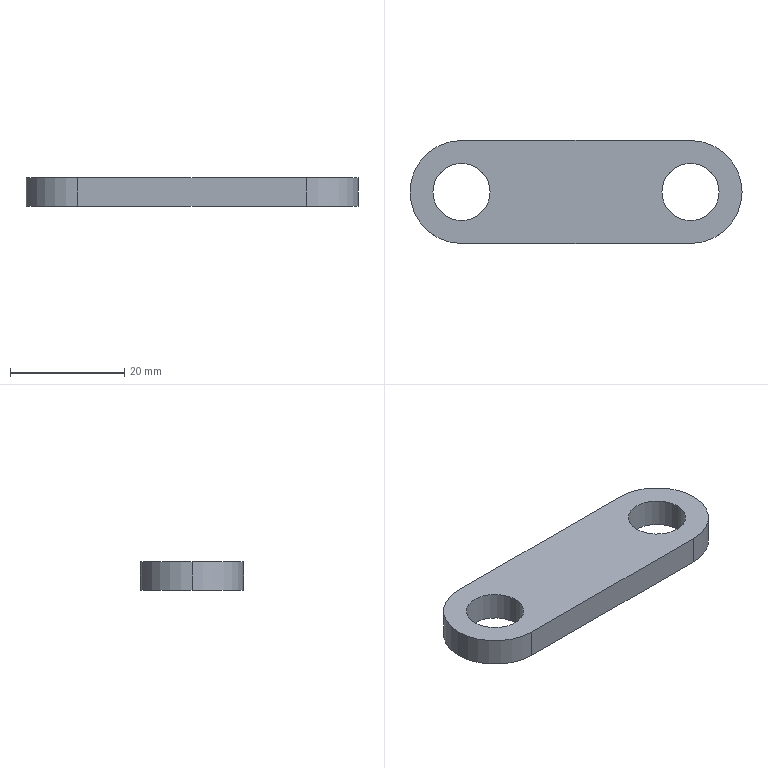Part | SolidWorks | features Cut 1, Extrusion 1 | 1 solid | 11 faces | box 58 x 18 x 5 mm | volume 4087 mm3 | cylinder 7 | plane 4 | commonest cylinder face diameters 10 x4 18 x3
STEP:
#1=CARTESIAN_POINT('',(35.,0.,0.));
#2=VERTEX_POINT('',#1);
#3=CARTESIAN_POINT('',(45.,0.,0.));
#4=VERTEX_POINT('',#3);
#5=CARTESIAN_POINT('',(40.,0.,0.));
#6=DIRECTION('',(0.,0.,1.));
#7=DIRECTION('',(1.,0.,0.));
#8=AXIS2_PLACEMENT_3D('',#5,#6,#7);
#9=CIRCLE('',#8,5.);
#10=EDGE_CURVE('',#2,#4,#9,.T.);
#11=ORIENTED_EDGE('',*,*,#10,.F.);
#12=CARTESIAN_POINT('',(35.,0.,5.));
#13=VERTEX_POINT('',#12);
#14=CARTESIAN_POINT('',(35.,0.,0.));
#15=DIRECTION('',(0.,0.,1.));
#16=VECTOR('',#15,1000.);
#17=LINE('',#14,#16);
#18=EDGE_CURVE('',#2,#13,#17,.T.);
#19=ORIENTED_EDGE('',*,*,#18,.T.);
#20=CARTESIAN_POINT('',(45.,0.,5.));
#21=VERTEX_POINT('',#20);
#22=CARTESIAN_POINT('',(40.,0.,5.));
#23=DIRECTION('',(0.,0.,1.));
#24=DIRECTION('',(1.,0.,0.));
#25=AXIS2_PLACEMENT_3D('',#22,#23,#24);
#26=CIRCLE('',#25,5.);
#27=EDGE_CURVE('',#13,#21,#26,.T.);
#28=ORIENTED_EDGE('',*,*,#27,.T.);
#29=CARTESIAN_POINT('',(45.,0.,0.));
#30=DIRECTION('',(0.,0.,1.));
#31=VECTOR('',#30,1000.);
#32=LINE('',#29,#31);
#33=EDGE_CURVE('',#4,#21,#32,.T.);
#34=ORIENTED_EDGE('',*,*,#33,.F.);
#35=EDGE_LOOP('',(#11,#19,#28,#34));
#36=FACE_OUTER_BOUND('',#35,.T.);
#37=CARTESIAN_POINT('',(40.,0.,0.));
#38=DIRECTION('',(0.,0.,1.));
#39=DIRECTION('',(1.,0.,0.));
#40=AXIS2_PLACEMENT_3D('',#37,#38,#39);
#41=CYLINDRICAL_SURFACE('',#40,5.);
#42=ADVANCED_FACE('',(#36),#41,.F.);
#43=CARTESIAN_POINT('',(-5.,0.,0.));
#44=VERTEX_POINT('',#43);
#45=CARTESIAN_POINT('',(5.,0.,0.));
#46=VERTEX_POINT('',#45);
#47=CARTESIAN_POINT('',(0.,0.,0.));
#48=DIRECTION('',(0.,0.,1.));
#49=DIRECTION('',(1.,0.,0.));
#50=AXIS2_PLACEMENT_3D('',#47,#48,#49);
#51=CIRCLE('',#50,5.);
#52=EDGE_CURVE('',#44,#46,#51,.T.);
#53=ORIENTED_EDGE('',*,*,#52,.F.);
#54=CARTESIAN_POINT('',(-5.,0.,5.));
#55=VERTEX_POINT('',#54);
#56=CARTESIAN_POINT('',(-5.,0.,0.));
#57=DIRECTION('',(0.,0.,1.));
#58=VECTOR('',#57,1000.);
#59=LINE('',#56,#58);
#60=EDGE_CURVE('',#44,#55,#59,.T.);
#61=ORIENTED_EDGE('',*,*,#60,.T.);
#62=CARTESIAN_POINT('',(5.,0.,5.));
#63=VERTEX_POINT('',#62);
#64=CARTESIAN_POINT('',(0.,0.,5.));
#65=DIRECTION('',(0.,0.,1.));
#66=DIRECTION('',(1.,0.,0.));
#67=AXIS2_PLACEMENT_3D('',#64,#65,#66);
#68=CIRCLE('',#67,5.);
#69=EDGE_CURVE('',#55,#63,#68,.T.);
#70=ORIENTED_EDGE('',*,*,#69,.T.);
#71=CARTESIAN_POINT('',(5.,0.,0.));
#72=DIRECTION('',(0.,0.,1.));
#73=VECTOR('',#72,1000.);
#74=LINE('',#71,#73);
#75=EDGE_CURVE('',#46,#63,#74,.T.);
#76=ORIENTED_EDGE('',*,*,#75,.F.);
#77=EDGE_LOOP('',(#53,#61,#70,#76));
#78=FACE_OUTER_BOUND('',#77,.T.);
#79=CARTESIAN_POINT('',(0.,0.,0.));
#80=DIRECTION('',(0.,0.,1.));
#81=DIRECTION('',(1.,0.,0.));
#82=AXIS2_PLACEMENT_3D('',#79,#80,#81);
#83=CYLINDRICAL_SURFACE('',#82,5.);
#84=ADVANCED_FACE('',(#78),#83,.F.);
#85=CARTESIAN_POINT('',(-9.,0.,5.));
#86=VERTEX_POINT('',#85);
#87=CARTESIAN_POINT('',(0.,-9.,5.));
#88=VERTEX_POINT('',#87);
#89=CARTESIAN_POINT('',(0.,0.,5.));
#90=DIRECTION('',(0.,0.,1.));
#91=DIRECTION('',(1.,0.,0.));
#92=AXIS2_PLACEMENT_3D('',#89,#90,#91);
#93=CIRCLE('',#92,9.);
#94=EDGE_CURVE('',#86,#88,#93,.T.);
#95=ORIENTED_EDGE('',*,*,#94,.F.);
#96=CARTESIAN_POINT('',(-9.,0.,0.));
#97=VERTEX_POINT('',#96);
#98=CARTESIAN_POINT('',(-9.,0.,5.));
#99=DIRECTION('',(0.,0.,-1.));
#100=VECTOR('',#99,1000.);
#101=LINE('',#98,#100);
#102=EDGE_CURVE('',#86,#97,#101,.T.);
#103=ORIENTED_EDGE('',*,*,#102,.T.);
#104=CARTESIAN_POINT('',(0.,-9.,0.));
#105=VERTEX_POINT('',#104);
#106=CARTESIAN_POINT('',(0.,0.,0.));
#107=DIRECTION('',(0.,0.,1.));
#108=DIRECTION('',(1.,0.,0.));
#109=AXIS2_PLACEMENT_3D('',#106,#107,#108);
#110=CIRCLE('',#109,9.);
#111=EDGE_CURVE('',#97,#105,#110,.T.);
#112=ORIENTED_EDGE('',*,*,#111,.T.);
#113=CARTESIAN_POINT('',(0.,-9.,5.));
#114=DIRECTION('',(0.,0.,-1.));
#115=VECTOR('',#114,1000.);
#116=LINE('',#113,#115);
#117=EDGE_CURVE('',#88,#105,#116,.T.);
#118=ORIENTED_EDGE('',*,*,#117,.F.);
#119=EDGE_LOOP('',(#95,#103,#112,#118));
#120=FACE_OUTER_BOUND('',#119,.T.);
#121=CARTESIAN_POINT('',(0.,0.,5.));
#122=DIRECTION('',(0.,0.,-1.));
#123=DIRECTION('',(-1.,0.,0.));
#124=AXIS2_PLACEMENT_3D('',#121,#122,#123);
#125=CYLINDRICAL_SURFACE('',#124,9.);
#126=ADVANCED_FACE('',(#120),#125,.T.);
#127=ORIENTED_EDGE('',*,*,#102,.F.);
#128=CARTESIAN_POINT('',(0.,9.,5.));
#129=VERTEX_POINT('',#128);
#130=CARTESIAN_POINT('',(0.,0.,5.));
#131=DIRECTION('',(0.,0.,1.));
#132=DIRECTION('',(1.,0.,0.));
#133=AXIS2_PLACEMENT_3D('',#130,#131,#132);
#134=CIRCLE('',#133,9.);
#135=EDGE_CURVE('',#129,#86,#134,.T.);
#136=ORIENTED_EDGE('',*,*,#135,.F.);
#137=CARTESIAN_POINT('',(0.,9.,0.));
#138=VERTEX_POINT('',#137);
#139=CARTESIAN_POINT('',(0.,9.,5.));
#140=DIRECTION('',(0.,0.,-1.));
#141=VECTOR('',#140,1000.);
#142=LINE('',#139,#141);
#143=EDGE_CURVE('',#129,#138,#142,.T.);
#144=ORIENTED_EDGE('',*,*,#143,.T.);
#145=CARTESIAN_POINT('',(0.,0.,0.));
#146=DIRECTION('',(0.,0.,1.));
#147=DIRECTION('',(1.,0.,0.));
#148=AXIS2_PLACEMENT_3D('',#145,#146,#147);
#149=CIRCLE('',#148,9.);
#150=EDGE_CURVE('',#138,#97,#149,.T.);
#151=ORIENTED_EDGE('',*,*,#150,.T.);
#152=EDGE_LOOP('',(#127,#136,#144,#151));
#153=FACE_OUTER_BOUND('',#152,.T.);
#154=CARTESIAN_POINT('',(0.,0.,5.));
#155=DIRECTION('',(0.,0.,-1.));
#156=DIRECTION('',(-1.,0.,0.));
#157=AXIS2_PLACEMENT_3D('',#154,#155,#156);
#158=CYLINDRICAL_SURFACE('',#157,9.);
#159=ADVANCED_FACE('',(#153),#158,.T.);
#160=CARTESIAN_POINT('',(40.,-9.,0.));
#161=VERTEX_POINT('',#160);
#162=CARTESIAN_POINT('',(0.,-9.,0.));
#163=DIRECTION('',(1.,0.,0.));
#164=VECTOR('',#163,1000.);
#165=LINE('',#162,#164);
#166=EDGE_CURVE('',#105,#161,#165,.T.);
#167=ORIENTED_EDGE('',*,*,#166,.T.);
#168=CARTESIAN_POINT('',(40.,-9.,5.));
#169=VERTEX_POINT('',#168);
#170=CARTESIAN_POINT('',(40.,-9.,5.));
#171=DIRECTION('',(0.,0.,-1.));
#172=VECTOR('',#171,1000.);
#173=LINE('',#170,#172);
#174=EDGE_CURVE('',#169,#161,#173,.T.);
#175=ORIENTED_EDGE('',*,*,#174,.F.);
#176=CARTESIAN_POINT('',(0.,-9.,5.));
#177=DIRECTION('',(1.,0.,0.));
#178=VECTOR('',#177,1000.);
#179=LINE('',#176,#178);
#180=EDGE_CURVE('',#88,#169,#179,.T.);
#181=ORIENTED_EDGE('',*,*,#180,.F.);
#182=ORIENTED_EDGE('',*,*,#117,.T.);
#183=EDGE_LOOP('',(#167,#175,#181,#182));
#184=FACE_OUTER_BOUND('',#183,.T.);
#185=CARTESIAN_POINT('',(0.,-9.,5.));
#186=DIRECTION('',(0.,1.,0.));
#187=DIRECTION('',(0.,0.,1.));
#188=AXIS2_PLACEMENT_3D('',#185,#186,#187);
#189=PLANE('',#188);
#190=ADVANCED_FACE('',(#184),#189,.F.);
#191=CARTESIAN_POINT('',(40.,9.,0.));
#192=VERTEX_POINT('',#191);
#193=CARTESIAN_POINT('',(40.,0.,0.));
#194=DIRECTION('',(0.,0.,1.));
#195=DIRECTION('',(1.,0.,0.));
#196=AXIS2_PLACEMENT_3D('',#193,#194,#195);
#197=CIRCLE('',#196,9.);
#198=EDGE_CURVE('',#161,#192,#197,.T.);
#199=ORIENTED_EDGE('',*,*,#198,.T.);
#200=CARTESIAN_POINT('',(40.,9.,5.));
#201=VERTEX_POINT('',#200);
#202=CARTESIAN_POINT('',(40.,9.,5.));
#203=DIRECTION('',(0.,0.,-1.));
#204=VECTOR('',#203,1000.);
#205=LINE('',#202,#204);
#206=EDGE_CURVE('',#201,#192,#205,.T.);
#207=ORIENTED_EDGE('',*,*,#206,.F.);
#208=CARTESIAN_POINT('',(40.,0.,5.));
#209=DIRECTION('',(0.,0.,1.));
#210=DIRECTION('',(1.,0.,0.));
#211=AXIS2_PLACEMENT_3D('',#208,#209,#210);
#212=CIRCLE('',#211,9.);
#213=EDGE_CURVE('',#169,#201,#212,.T.);
#214=ORIENTED_EDGE('',*,*,#213,.F.);
#215=ORIENTED_EDGE('',*,*,#174,.T.);
#216=EDGE_LOOP('',(#199,#207,#214,#215));
#217=FACE_OUTER_BOUND('',#216,.T.);
#218=CARTESIAN_POINT('',(40.,0.,5.));
#219=DIRECTION('',(0.,0.,-1.));
#220=DIRECTION('',(-1.,0.,0.));
#221=AXIS2_PLACEMENT_3D('',#218,#219,#220);
#222=CYLINDRICAL_SURFACE('',#221,9.);
#223=ADVANCED_FACE('',(#217),#222,.T.);
#224=CARTESIAN_POINT('',(0.,9.,0.));
#225=DIRECTION('',(-1.,0.,0.));
#226=VECTOR('',#225,1000.);
#227=LINE('',#224,#226);
#228=EDGE_CURVE('',#192,#138,#227,.T.);
#229=ORIENTED_EDGE('',*,*,#228,.T.);
#230=ORIENTED_EDGE('',*,*,#143,.F.);
#231=CARTESIAN_POINT('',(0.,9.,5.));
#232=DIRECTION('',(-1.,0.,0.));
#233=VECTOR('',#232,1000.);
#234=LINE('',#231,#233);
#235=EDGE_CURVE('',#201,#129,#234,.T.);
#236=ORIENTED_EDGE('',*,*,#235,.F.);
#237=ORIENTED_EDGE('',*,*,#206,.T.);
#238=EDGE_LOOP('',(#229,#230,#236,#237));
#239=FACE_OUTER_BOUND('',#238,.T.);
#240=CARTESIAN_POINT('',(0.,9.,5.));
#241=DIRECTION('',(0.,-1.,0.));
#242=DIRECTION('',(0.,0.,-1.));
#243=AXIS2_PLACEMENT_3D('',#240,#241,#242);
#244=PLANE('',#243);
#245=ADVANCED_FACE('',(#239),#244,.F.);
#246=CARTESIAN_POINT('',(40.,0.,5.));
#247=DIRECTION('',(0.,0.,1.));
#248=DIRECTION('',(1.,0.,0.));
#249=AXIS2_PLACEMENT_3D('',#246,#247,#248);
#250=CIRCLE('',#249,5.);
#251=EDGE_CURVE('',#21,#13,#250,.T.);
#252=ORIENTED_EDGE('',*,*,#251,.F.);
#253=ORIENTED_EDGE('',*,*,#27,.F.);
#254=EDGE_LOOP('',(#252,#253));
#255=FACE_BOUND('',#254,.T.);
#256=CARTESIAN_POINT('',(0.,0.,5.));
#257=DIRECTION('',(0.,0.,1.));
#258=DIRECTION('',(1.,0.,0.));
#259=AXIS2_PLACEMENT_3D('',#256,#257,#258);
#260=CIRCLE('',#259,5.);
#261=EDGE_CURVE('',#63,#55,#260,.T.);
#262=ORIENTED_EDGE('',*,*,#261,.F.);
#263=ORIENTED_EDGE('',*,*,#69,.F.);
#264=EDGE_LOOP('',(#262,#263));
#265=FACE_BOUND('',#264,.T.);
#266=ORIENTED_EDGE('',*,*,#135,.T.);
#267=ORIENTED_EDGE('',*,*,#94,.T.);
#268=ORIENTED_EDGE('',*,*,#180,.T.);
#269=ORIENTED_EDGE('',*,*,#213,.T.);
#270=ORIENTED_EDGE('',*,*,#235,.T.);
#271=EDGE_LOOP('',(#266,#267,#268,#269,#270));
#272=FACE_OUTER_BOUND('',#271,.T.);
#273=CARTESIAN_POINT('',(0.,0.,5.));
#274=DIRECTION('',(0.,0.,1.));
#275=DIRECTION('',(1.,0.,0.));
#276=AXIS2_PLACEMENT_3D('',#273,#274,#275);
#277=PLANE('',#276);
#278=ADVANCED_FACE('',(#255,#265,#272),#277,.T.);
#279=CARTESIAN_POINT('',(40.,0.,0.));
#280=DIRECTION('',(0.,0.,1.));
#281=DIRECTION('',(1.,0.,0.));
#282=AXIS2_PLACEMENT_3D('',#279,#280,#281);
#283=CIRCLE('',#282,5.);
#284=EDGE_CURVE('',#4,#2,#283,.T.);
#285=ORIENTED_EDGE('',*,*,#284,.T.);
#286=ORIENTED_EDGE('',*,*,#10,.T.);
#287=EDGE_LOOP('',(#285,#286));
#288=FACE_BOUND('',#287,.T.);
#289=CARTESIAN_POINT('',(0.,0.,0.));
#290=DIRECTION('',(0.,0.,1.));
#291=DIRECTION('',(1.,0.,0.));
#292=AXIS2_PLACEMENT_3D('',#289,#290,#291);
#293=CIRCLE('',#292,5.);
#294=EDGE_CURVE('',#46,#44,#293,.T.);
#295=ORIENTED_EDGE('',*,*,#294,.T.);
#296=ORIENTED_EDGE('',*,*,#52,.T.);
#297=EDGE_LOOP('',(#295,#296));
#298=FACE_BOUND('',#297,.T.);
#299=ORIENTED_EDGE('',*,*,#150,.F.);
#300=ORIENTED_EDGE('',*,*,#228,.F.);
#301=ORIENTED_EDGE('',*,*,#198,.F.);
#302=ORIENTED_EDGE('',*,*,#166,.F.);
#303=ORIENTED_EDGE('',*,*,#111,.F.);
#304=EDGE_LOOP('',(#299,#300,#301,#302,#303));
#305=FACE_OUTER_BOUND('',#304,.T.);
#306=CARTESIAN_POINT('',(0.,0.,0.));
#307=DIRECTION('',(0.,0.,1.));
#308=DIRECTION('',(1.,0.,0.));
#309=AXIS2_PLACEMENT_3D('',#306,#307,#308);
#310=PLANE('',#309);
#311=ADVANCED_FACE('',(#288,#298,#305),#310,.F.);
#312=ORIENTED_EDGE('',*,*,#60,.F.);
#313=ORIENTED_EDGE('',*,*,#294,.F.);
#314=ORIENTED_EDGE('',*,*,#75,.T.);
#315=ORIENTED_EDGE('',*,*,#261,.T.);
#316=EDGE_LOOP('',(#312,#313,#314,#315));
#317=FACE_OUTER_BOUND('',#316,.T.);
#318=CARTESIAN_POINT('',(0.,0.,0.));
#319=DIRECTION('',(0.,0.,1.));
#320=DIRECTION('',(1.,0.,0.));
#321=AXIS2_PLACEMENT_3D('',#318,#319,#320);
#322=CYLINDRICAL_SURFACE('',#321,5.);
#323=ADVANCED_FACE('',(#317),#322,.F.);
#324=ORIENTED_EDGE('',*,*,#18,.F.);
#325=ORIENTED_EDGE('',*,*,#284,.F.);
#326=ORIENTED_EDGE('',*,*,#33,.T.);
#327=ORIENTED_EDGE('',*,*,#251,.T.);
#328=EDGE_LOOP('',(#324,#325,#326,#327));
#329=FACE_OUTER_BOUND('',#328,.T.);
#330=CARTESIAN_POINT('',(40.,0.,0.));
#331=DIRECTION('',(0.,0.,1.));
#332=DIRECTION('',(1.,0.,0.));
#333=AXIS2_PLACEMENT_3D('',#330,#331,#332);
#334=CYLINDRICAL_SURFACE('',#333,5.);
#335=ADVANCED_FACE('',(#329),#334,.F.);
#336=CLOSED_SHELL('',(#42,#84,#126,#159,#190,#223,#245,#278,#311,#323,#335));
#337=MANIFOLD_SOLID_BREP('',#336);
#338=CARTESIAN_POINT('',(0.,0.,0.));
#339=DIRECTION('',(0.,0.,1.));
#340=DIRECTION('',(1.,0.,0.));
#341=AXIS2_PLACEMENT_3D('',#338,#339,#340);
#342=(LENGTH_UNIT()NAMED_UNIT(*)SI_UNIT(.MILLI.,.METRE.));
#343=UNCERTAINTY_MEASURE_WITH_UNIT(LENGTH_MEASURE(0.00001),#342,'','');
#344=(NAMED_UNIT(*)PLANE_ANGLE_UNIT()SI_UNIT($,.RADIAN.));
#345=(NAMED_UNIT(*)SI_UNIT($,.STERADIAN.)SOLID_ANGLE_UNIT());
#346=(GEOMETRIC_REPRESENTATION_CONTEXT(3)GLOBAL_UNCERTAINTY_ASSIGNED_CONTEXT((#343))GLOBAL_UNIT_ASSIGNED_CONTEXT((#342,#344,#345))REPRESENTATION_CONTEXT('',''));
#347=ADVANCED_BREP_SHAPE_REPRESENTATION('',(#337,#341),#346);